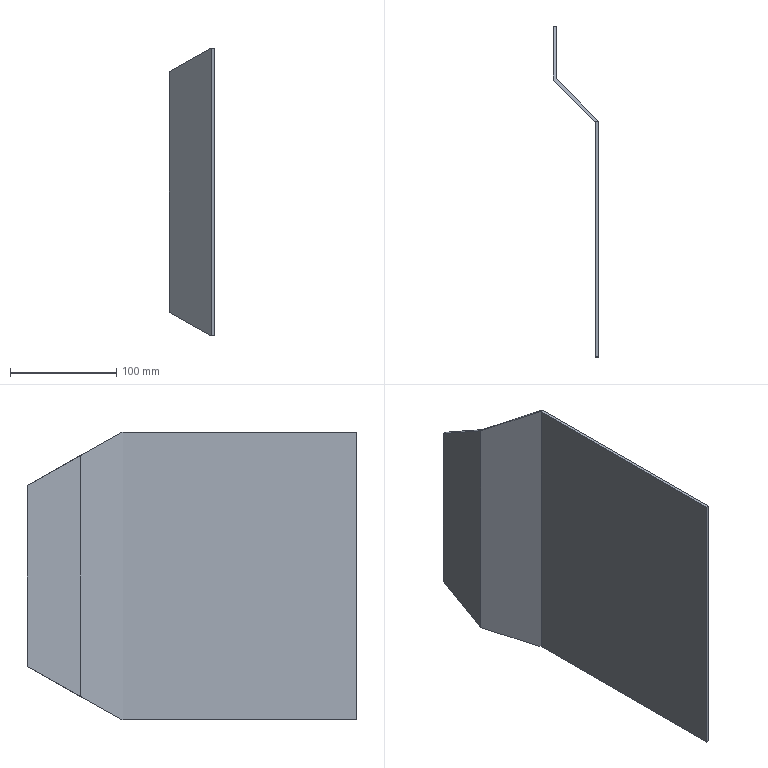Part | SolidWorks | features Extrusion 1, ICE 1 | 1 solid | 12 faces | box 43 x 310 x 270 mm | volume 250121 mm3 | plane 12
STEP:
#1=CARTESIAN_POINT('',(3.,0.,220.));
#2=VERTEX_POINT('',#1);
#3=CARTESIAN_POINT('',(3.,0.,50.));
#4=VERTEX_POINT('',#3);
#5=CARTESIAN_POINT('',(3.,0.,270.));
#6=DIRECTION('',(0.,0.,-1.));
#7=VECTOR('',#6,1000.);
#8=LINE('',#5,#7);
#9=EDGE_CURVE('',#2,#4,#8,.T.);
#10=ORIENTED_EDGE('',*,*,#9,.T.);
#11=CARTESIAN_POINT('',(0.,0.,50.));
#12=VERTEX_POINT('',#11);
#13=CARTESIAN_POINT('',(-227.,0.,50.));
#14=DIRECTION('',(1.,0.,0.));
#15=VECTOR('',#14,1000.);
#16=LINE('',#13,#15);
#17=EDGE_CURVE('',#12,#4,#16,.T.);
#18=ORIENTED_EDGE('',*,*,#17,.F.);
#19=CARTESIAN_POINT('',(0.,0.,220.));
#20=VERTEX_POINT('',#19);
#21=CARTESIAN_POINT('',(0.,0.,270.));
#22=DIRECTION('',(0.,0.,-1.));
#23=VECTOR('',#22,1000.);
#24=LINE('',#21,#23);
#25=EDGE_CURVE('',#20,#12,#24,.T.);
#26=ORIENTED_EDGE('',*,*,#25,.F.);
#27=CARTESIAN_POINT('',(-227.,0.,220.));
#28=DIRECTION('',(1.,0.,0.));
#29=VECTOR('',#28,1000.);
#30=LINE('',#27,#29);
#31=EDGE_CURVE('',#20,#2,#30,.T.);
#32=ORIENTED_EDGE('',*,*,#31,.T.);
#33=EDGE_LOOP('',(#10,#18,#26,#32));
#34=FACE_OUTER_BOUND('',#33,.T.);
#35=CARTESIAN_POINT('',(0.,0.,270.));
#36=DIRECTION('',(0.,-1.,0.));
#37=DIRECTION('',(0.,0.,-1.));
#38=AXIS2_PLACEMENT_3D('',#35,#36,#37);
#39=PLANE('',#38);
#40=ADVANCED_FACE('',(#34),#39,.F.);
#41=ORIENTED_EDGE('',*,*,#25,.T.);
#42=CARTESIAN_POINT('',(0.,-50.,21.833));
#43=VERTEX_POINT('',#42);
#44=CARTESIAN_POINT('',(0.,94.078,102.997));
#45=DIRECTION('',(0.,-0.8713,-0.4908));
#46=VECTOR('',#45,1000.);
#47=LINE('',#44,#46);
#48=EDGE_CURVE('',#12,#43,#47,.T.);
#49=ORIENTED_EDGE('',*,*,#48,.T.);
#50=CARTESIAN_POINT('',(0.,-50.,248.167));
#51=VERTEX_POINT('',#50);
#52=CARTESIAN_POINT('',(0.,-50.,270.));
#53=DIRECTION('',(0.,0.,-1.));
#54=VECTOR('',#53,1000.);
#55=LINE('',#52,#54);
#56=EDGE_CURVE('',#51,#43,#55,.T.);
#57=ORIENTED_EDGE('',*,*,#56,.F.);
#58=CARTESIAN_POINT('',(0.,-21.381,232.045));
#59=DIRECTION('',(0.,0.8713,-0.4908));
#60=VECTOR('',#59,1000.);
#61=LINE('',#58,#60);
#62=EDGE_CURVE('',#51,#20,#61,.T.);
#63=ORIENTED_EDGE('',*,*,#62,.T.);
#64=EDGE_LOOP('',(#41,#49,#57,#63));
#65=FACE_OUTER_BOUND('',#64,.T.);
#66=CARTESIAN_POINT('',(0.,0.,270.));
#67=DIRECTION('',(1.,0.,0.));
#68=DIRECTION('',(0.,1.,0.));
#69=AXIS2_PLACEMENT_3D('',#66,#67,#68);
#70=PLANE('',#69);
#71=ADVANCED_FACE('',(#65),#70,.F.);
#72=ORIENTED_EDGE('',*,*,#56,.T.);
#73=CARTESIAN_POINT('',(38.757,-88.757,0.));
#74=VERTEX_POINT('',#73);
#75=CARTESIAN_POINT('',(-25.806,-24.194,36.371));
#76=DIRECTION('',(0.6569,-0.6569,-0.3701));
#77=VECTOR('',#76,1000.);
#78=LINE('',#75,#77);
#79=EDGE_CURVE('',#43,#74,#78,.T.);
#80=ORIENTED_EDGE('',*,*,#79,.T.);
#81=CARTESIAN_POINT('',(40.,-90.,0.));
#82=VERTEX_POINT('',#81);
#83=CARTESIAN_POINT('',(40.,-90.,0.));
#84=DIRECTION('',(0.7071,-0.7071,0.));
#85=VECTOR('',#84,1000.);
#86=LINE('',#83,#85);
#87=EDGE_CURVE('',#74,#82,#86,.T.);
#88=ORIENTED_EDGE('',*,*,#87,.T.);
#89=CARTESIAN_POINT('',(40.,-90.,270.));
#90=VERTEX_POINT('',#89);
#91=CARTESIAN_POINT('',(40.,-90.,270.));
#92=DIRECTION('',(0.,0.,-1.));
#93=VECTOR('',#92,1000.);
#94=LINE('',#91,#93);
#95=EDGE_CURVE('',#90,#82,#94,.T.);
#96=ORIENTED_EDGE('',*,*,#95,.F.);
#97=CARTESIAN_POINT('',(38.757,-88.757,270.));
#98=VERTEX_POINT('',#97);
#99=CARTESIAN_POINT('',(40.,-90.,270.));
#100=DIRECTION('',(0.7071,-0.7071,0.));
#101=VECTOR('',#100,1000.);
#102=LINE('',#99,#101);
#103=EDGE_CURVE('',#98,#90,#102,.T.);
#104=ORIENTED_EDGE('',*,*,#103,.F.);
#105=CARTESIAN_POINT('',(39.83,-89.83,270.604));
#106=DIRECTION('',(-0.6569,0.6569,-0.3701));
#107=VECTOR('',#106,1000.);
#108=LINE('',#105,#107);
#109=EDGE_CURVE('',#98,#51,#108,.T.);
#110=ORIENTED_EDGE('',*,*,#109,.T.);
#111=EDGE_LOOP('',(#72,#80,#88,#96,#104,#110));
#112=FACE_OUTER_BOUND('',#111,.T.);
#113=CARTESIAN_POINT('',(40.,-90.,270.));
#114=DIRECTION('',(0.7071,0.7071,0.));
#115=DIRECTION('',(-0.7071,0.7071,0.));
#116=AXIS2_PLACEMENT_3D('',#113,#114,#115);
#117=PLANE('',#116);
#118=ADVANCED_FACE('',(#112),#117,.F.);
#119=CARTESIAN_POINT('',(40.,-310.,0.));
#120=VERTEX_POINT('',#119);
#121=CARTESIAN_POINT('',(40.,-90.,0.));
#122=DIRECTION('',(0.,-1.,0.));
#123=VECTOR('',#122,1000.);
#124=LINE('',#121,#123);
#125=EDGE_CURVE('',#82,#120,#124,.T.);
#126=ORIENTED_EDGE('',*,*,#125,.T.);
#127=CARTESIAN_POINT('',(40.,-310.,270.));
#128=VERTEX_POINT('',#127);
#129=CARTESIAN_POINT('',(40.,-310.,270.));
#130=DIRECTION('',(0.,0.,-1.));
#131=VECTOR('',#130,1000.);
#132=LINE('',#129,#131);
#133=EDGE_CURVE('',#128,#120,#132,.T.);
#134=ORIENTED_EDGE('',*,*,#133,.F.);
#135=CARTESIAN_POINT('',(40.,-90.,270.));
#136=DIRECTION('',(0.,-1.,0.));
#137=VECTOR('',#136,1000.);
#138=LINE('',#135,#137);
#139=EDGE_CURVE('',#90,#128,#138,.T.);
#140=ORIENTED_EDGE('',*,*,#139,.F.);
#141=ORIENTED_EDGE('',*,*,#95,.T.);
#142=EDGE_LOOP('',(#126,#134,#140,#141));
#143=FACE_OUTER_BOUND('',#142,.T.);
#144=CARTESIAN_POINT('',(40.,-90.,270.));
#145=DIRECTION('',(1.,0.,0.));
#146=DIRECTION('',(0.,1.,0.));
#147=AXIS2_PLACEMENT_3D('',#144,#145,#146);
#148=PLANE('',#147);
#149=ADVANCED_FACE('',(#143),#148,.F.);
#150=CARTESIAN_POINT('',(43.,-310.,0.));
#151=VERTEX_POINT('',#150);
#152=CARTESIAN_POINT('',(40.,-310.,0.));
#153=DIRECTION('',(1.,0.,0.));
#154=VECTOR('',#153,1000.);
#155=LINE('',#152,#154);
#156=EDGE_CURVE('',#120,#151,#155,.T.);
#157=ORIENTED_EDGE('',*,*,#156,.T.);
#158=CARTESIAN_POINT('',(43.,-310.,270.));
#159=VERTEX_POINT('',#158);
#160=CARTESIAN_POINT('',(43.,-310.,270.));
#161=DIRECTION('',(0.,0.,-1.));
#162=VECTOR('',#161,1000.);
#163=LINE('',#160,#162);
#164=EDGE_CURVE('',#159,#151,#163,.T.);
#165=ORIENTED_EDGE('',*,*,#164,.F.);
#166=CARTESIAN_POINT('',(40.,-310.,270.));
#167=DIRECTION('',(1.,0.,0.));
#168=VECTOR('',#167,1000.);
#169=LINE('',#166,#168);
#170=EDGE_CURVE('',#128,#159,#169,.T.);
#171=ORIENTED_EDGE('',*,*,#170,.F.);
#172=ORIENTED_EDGE('',*,*,#133,.T.);
#173=EDGE_LOOP('',(#157,#165,#171,#172));
#174=FACE_OUTER_BOUND('',#173,.T.);
#175=CARTESIAN_POINT('',(40.,-310.,270.));
#176=DIRECTION('',(0.,1.,0.));
#177=DIRECTION('',(0.,0.,1.));
#178=AXIS2_PLACEMENT_3D('',#175,#176,#177);
#179=PLANE('',#178);
#180=ADVANCED_FACE('',(#174),#179,.F.);
#181=CARTESIAN_POINT('',(43.,-88.757,0.));
#182=VERTEX_POINT('',#181);
#183=CARTESIAN_POINT('',(43.,-88.757,0.));
#184=DIRECTION('',(0.,1.,0.));
#185=VECTOR('',#184,1000.);
#186=LINE('',#183,#185);
#187=EDGE_CURVE('',#151,#182,#186,.T.);
#188=ORIENTED_EDGE('',*,*,#187,.T.);
#189=CARTESIAN_POINT('',(43.,-88.757,270.));
#190=VERTEX_POINT('',#189);
#191=CARTESIAN_POINT('',(43.,-88.757,270.));
#192=DIRECTION('',(0.,0.,-1.));
#193=VECTOR('',#192,1000.);
#194=LINE('',#191,#193);
#195=EDGE_CURVE('',#190,#182,#194,.T.);
#196=ORIENTED_EDGE('',*,*,#195,.F.);
#197=CARTESIAN_POINT('',(43.,-88.757,270.));
#198=DIRECTION('',(0.,1.,0.));
#199=VECTOR('',#198,1000.);
#200=LINE('',#197,#199);
#201=EDGE_CURVE('',#159,#190,#200,.T.);
#202=ORIENTED_EDGE('',*,*,#201,.F.);
#203=ORIENTED_EDGE('',*,*,#164,.T.);
#204=EDGE_LOOP('',(#188,#196,#202,#203));
#205=FACE_OUTER_BOUND('',#204,.T.);
#206=CARTESIAN_POINT('',(43.,-88.757,270.));
#207=DIRECTION('',(-1.,0.,0.));
#208=DIRECTION('',(0.,0.,1.));
#209=AXIS2_PLACEMENT_3D('',#206,#207,#208);
#210=PLANE('',#209);
#211=ADVANCED_FACE('',(#205),#210,.F.);
#212=ORIENTED_EDGE('',*,*,#195,.T.);
#213=CARTESIAN_POINT('',(3.,-48.757,22.533));
#214=VERTEX_POINT('',#213);
#215=CARTESIAN_POINT('',(-22.635,-23.122,36.975));
#216=DIRECTION('',(-0.6569,0.6569,0.3701));
#217=VECTOR('',#216,1000.);
#218=LINE('',#215,#217);
#219=EDGE_CURVE('',#182,#214,#218,.T.);
#220=ORIENTED_EDGE('',*,*,#219,.T.);
#221=CARTESIAN_POINT('',(3.,-48.757,247.467));
#222=VERTEX_POINT('',#221);
#223=CARTESIAN_POINT('',(3.,-48.757,270.));
#224=DIRECTION('',(0.,0.,-1.));
#225=VECTOR('',#224,1000.);
#226=LINE('',#223,#225);
#227=EDGE_CURVE('',#222,#214,#226,.T.);
#228=ORIENTED_EDGE('',*,*,#227,.F.);
#229=CARTESIAN_POINT('',(43.,-88.757,270.));
#230=DIRECTION('',(0.6569,-0.6569,0.3701));
#231=VECTOR('',#230,1000.);
#232=LINE('',#229,#231);
#233=EDGE_CURVE('',#222,#190,#232,.T.);
#234=ORIENTED_EDGE('',*,*,#233,.T.);
#235=EDGE_LOOP('',(#212,#220,#228,#234));
#236=FACE_OUTER_BOUND('',#235,.T.);
#237=CARTESIAN_POINT('',(43.,-88.757,270.));
#238=DIRECTION('',(-0.7071,-0.7071,0.));
#239=DIRECTION('',(0.7071,-0.7071,0.));
#240=AXIS2_PLACEMENT_3D('',#237,#238,#239);
#241=PLANE('',#240);
#242=ADVANCED_FACE('',(#236),#241,.F.);
#243=ORIENTED_EDGE('',*,*,#227,.T.);
#244=CARTESIAN_POINT('',(3.,94.078,102.997));
#245=DIRECTION('',(0.,0.8713,0.4908));
#246=VECTOR('',#245,1000.);
#247=LINE('',#244,#246);
#248=EDGE_CURVE('',#214,#4,#247,.T.);
#249=ORIENTED_EDGE('',*,*,#248,.T.);
#250=ORIENTED_EDGE('',*,*,#9,.F.);
#251=CARTESIAN_POINT('',(3.,-21.381,232.045));
#252=DIRECTION('',(0.,-0.8713,0.4908));
#253=VECTOR('',#252,1000.);
#254=LINE('',#251,#253);
#255=EDGE_CURVE('',#2,#222,#254,.T.);
#256=ORIENTED_EDGE('',*,*,#255,.T.);
#257=EDGE_LOOP('',(#243,#249,#250,#256));
#258=FACE_OUTER_BOUND('',#257,.T.);
#259=CARTESIAN_POINT('',(3.,0.,270.));
#260=DIRECTION('',(-1.,0.,0.));
#261=DIRECTION('',(0.,-1.,0.));
#262=AXIS2_PLACEMENT_3D('',#259,#260,#261);
#263=PLANE('',#262);
#264=ADVANCED_FACE('',(#258),#263,.F.);
#265=ORIENTED_EDGE('',*,*,#201,.T.);
#266=CARTESIAN_POINT('',(0.,-88.757,270.));
#267=DIRECTION('',(-1.,0.,0.));
#268=VECTOR('',#267,1000.);
#269=LINE('',#266,#268);
#270=EDGE_CURVE('',#190,#98,#269,.T.);
#271=ORIENTED_EDGE('',*,*,#270,.T.);
#272=ORIENTED_EDGE('',*,*,#103,.T.);
#273=ORIENTED_EDGE('',*,*,#139,.T.);
#274=ORIENTED_EDGE('',*,*,#170,.T.);
#275=EDGE_LOOP('',(#265,#271,#272,#273,#274));
#276=FACE_OUTER_BOUND('',#275,.T.);
#277=CARTESIAN_POINT('',(0.,0.,270.));
#278=DIRECTION('',(0.,0.,-1.));
#279=DIRECTION('',(-1.,0.,0.));
#280=AXIS2_PLACEMENT_3D('',#277,#278,#279);
#281=PLANE('',#280);
#282=ADVANCED_FACE('',(#276),#281,.F.);
#283=CARTESIAN_POINT('',(0.,-88.757,0.));
#284=DIRECTION('',(-1.,0.,0.));
#285=VECTOR('',#284,1000.);
#286=LINE('',#283,#285);
#287=EDGE_CURVE('',#182,#74,#286,.T.);
#288=ORIENTED_EDGE('',*,*,#287,.F.);
#289=ORIENTED_EDGE('',*,*,#187,.F.);
#290=ORIENTED_EDGE('',*,*,#156,.F.);
#291=ORIENTED_EDGE('',*,*,#125,.F.);
#292=ORIENTED_EDGE('',*,*,#87,.F.);
#293=EDGE_LOOP('',(#288,#289,#290,#291,#292));
#294=FACE_OUTER_BOUND('',#293,.T.);
#295=CARTESIAN_POINT('',(0.,0.,0.));
#296=DIRECTION('',(0.,0.,-1.));
#297=DIRECTION('',(-1.,0.,0.));
#298=AXIS2_PLACEMENT_3D('',#295,#296,#297);
#299=PLANE('',#298);
#300=ADVANCED_FACE('',(#294),#299,.T.);
#301=ORIENTED_EDGE('',*,*,#109,.F.);
#302=ORIENTED_EDGE('',*,*,#270,.F.);
#303=ORIENTED_EDGE('',*,*,#233,.F.);
#304=ORIENTED_EDGE('',*,*,#255,.F.);
#305=ORIENTED_EDGE('',*,*,#31,.F.);
#306=ORIENTED_EDGE('',*,*,#62,.F.);
#307=EDGE_LOOP('',(#301,#302,#303,#304,#305,#306));
#308=FACE_OUTER_BOUND('',#307,.T.);
#309=CARTESIAN_POINT('',(-227.,0.,220.));
#310=DIRECTION('',(0.,-0.4908,-0.8713));
#311=DIRECTION('',(0.,0.8713,-0.4908));
#312=AXIS2_PLACEMENT_3D('',#309,#310,#311);
#313=PLANE('',#312);
#314=ADVANCED_FACE('',(#308),#313,.F.);
#315=ORIENTED_EDGE('',*,*,#17,.T.);
#316=ORIENTED_EDGE('',*,*,#248,.F.);
#317=ORIENTED_EDGE('',*,*,#219,.F.);
#318=ORIENTED_EDGE('',*,*,#287,.T.);
#319=ORIENTED_EDGE('',*,*,#79,.F.);
#320=ORIENTED_EDGE('',*,*,#48,.F.);
#321=EDGE_LOOP('',(#315,#316,#317,#318,#319,#320));
#322=FACE_OUTER_BOUND('',#321,.T.);
#323=CARTESIAN_POINT('',(-227.,0.,50.));
#324=DIRECTION('',(0.,-0.4908,0.8713));
#325=DIRECTION('',(0.,-0.8713,-0.4908));
#326=AXIS2_PLACEMENT_3D('',#323,#324,#325);
#327=PLANE('',#326);
#328=ADVANCED_FACE('',(#322),#327,.F.);
#329=CLOSED_SHELL('',(#40,#71,#118,#149,#180,#211,#242,#264,#282,#300,#314,#328));
#330=MANIFOLD_SOLID_BREP('',#329);
#331=CARTESIAN_POINT('',(0.,0.,0.));
#332=DIRECTION('',(0.,0.,1.));
#333=DIRECTION('',(1.,0.,0.));
#334=AXIS2_PLACEMENT_3D('',#331,#332,#333);
#335=(LENGTH_UNIT()NAMED_UNIT(*)SI_UNIT(.MILLI.,.METRE.));
#336=UNCERTAINTY_MEASURE_WITH_UNIT(LENGTH_MEASURE(0.00001),#335,'','');
#337=(NAMED_UNIT(*)PLANE_ANGLE_UNIT()SI_UNIT($,.RADIAN.));
#338=(NAMED_UNIT(*)SI_UNIT($,.STERADIAN.)SOLID_ANGLE_UNIT());
#339=(GEOMETRIC_REPRESENTATION_CONTEXT(3)GLOBAL_UNCERTAINTY_ASSIGNED_CONTEXT((#336))GLOBAL_UNIT_ASSIGNED_CONTEXT((#335,#337,#338))REPRESENTATION_CONTEXT('',''));
#340=ADVANCED_BREP_SHAPE_REPRESENTATION('',(#330,#334),#339);